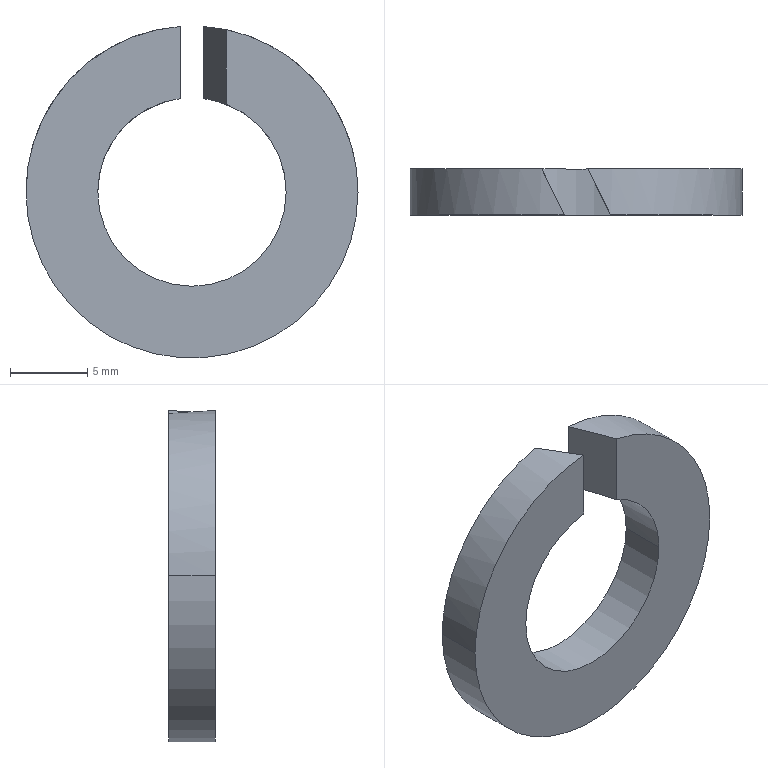Part | STEP file | ZZ24-M12 | 1 solid | 10 faces | box 21.5 x 3 x 21.473 mm | volume 696.301 mm3 | cylinder 6 | plane 4 | commonest cylinder face diameters 12.2 x3 21.5 x3
STEP:
#1=CARTESIAN_POINT('',(0.,0.,0.));
#2=DIRECTION('',(0.,0.,1.));
#3=DIRECTION('',(1.,0.,0.));
#4=AXIS2_PLACEMENT_3D('',#1,#2,#3);
#5=CARTESIAN_POINT('',(2.232,0.,5.677));
#6=VERTEX_POINT('',#5);
#7=CARTESIAN_POINT('',(0.7684,3.,6.051));
#8=VERTEX_POINT('',#7);
#9=CARTESIAN_POINT('',(2.232,0.,5.677));
#10=CARTESIAN_POINT('',(1.761,0.9656,5.862));
#11=CARTESIAN_POINT('',(1.27,1.971,5.988));
#12=CARTESIAN_POINT('',(0.7684,3.,6.051));
#13=(BOUNDED_CURVE()B_SPLINE_CURVE(3,(#9,#10,#11,#12),.UNSPECIFIED.,.F.,.F.)B_SPLINE_CURVE_WITH_KNOTS((4,4),(1.196,1.444),.PIECEWISE_BEZIER_KNOTS.)CURVE()GEOMETRIC_REPRESENTATION_ITEM()RATIONAL_B_SPLINE_CURVE((1.,0.9949,0.9949,1.))REPRESENTATION_ITEM(''));
#14=CARTESIAN_POINT('',(0.,3.,0.));
#15=DIRECTION('',(0.,-1.,0.));
#16=DIRECTION('',(-1.,0.,0.001512));
#17=AXIS2_PLACEMENT_3D('',#14,#15,#16);
#18=CYLINDRICAL_SURFACE('',#17,6.1);
#19=CARTESIAN_POINT('',(4.339,3.));
#20=CARTESIAN_POINT('',(4.343,2.956));
#21=CARTESIAN_POINT('',(4.351,2.869));
#22=CARTESIAN_POINT('',(4.362,2.737));
#23=CARTESIAN_POINT('',(4.373,2.604));
#24=CARTESIAN_POINT('',(4.384,2.471));
#25=CARTESIAN_POINT('',(4.396,2.337));
#26=CARTESIAN_POINT('',(4.407,2.203));
#27=CARTESIAN_POINT('',(4.418,2.068));
#28=CARTESIAN_POINT('',(4.43,1.933));
#29=CARTESIAN_POINT('',(4.441,1.797));
#30=CARTESIAN_POINT('',(4.452,1.661));
#31=CARTESIAN_POINT('',(4.463,1.524));
#32=CARTESIAN_POINT('',(4.475,1.387));
#33=CARTESIAN_POINT('',(4.486,1.249));
#34=CARTESIAN_POINT('',(4.497,1.112));
#35=CARTESIAN_POINT('',(4.509,0.9734));
#36=CARTESIAN_POINT('',(4.52,0.835));
#37=CARTESIAN_POINT('',(4.531,0.6964));
#38=CARTESIAN_POINT('',(4.543,0.5575));
#39=CARTESIAN_POINT('',(4.554,0.4183));
#40=CARTESIAN_POINT('',(4.565,0.2791));
#41=CARTESIAN_POINT('',(4.576,0.1396));
#42=CARTESIAN_POINT('',(4.584,0.04654));
#43=CARTESIAN_POINT('',(4.588,0.));
#44=B_SPLINE_CURVE_WITH_KNOTS('',3,(#19,#20,#21,#22,#23,#24,#25,#26,#27,#28,#29,#30,#31,#32,#33,#34,#35,#36,#37,#38,#39,#40,#41,#42,#43),.UNSPECIFIED.,.F.,.F.,(4,1,1,1,1,1,1,1,1,1,1,1,1,1,1,1,1,1,1,1,1,1,4),(1.196,1.208,1.219,1.23,1.241,1.253,1.264,1.275,1.287,1.298,1.309,1.32,1.332,1.343,1.354,1.366,1.377,1.388,1.399,1.411,1.422,1.433,1.444),.QUASI_UNIFORM_KNOTS.);
#45=(GEOMETRIC_REPRESENTATION_CONTEXT(2)PARAMETRIC_REPRESENTATION_CONTEXT()REPRESENTATION_CONTEXT('',''));
#46=DEFINITIONAL_REPRESENTATION('',(#44),#45);
#47=PCURVE('',#18,#46);
#48=CARTESIAN_POINT('',(2.232,0.,10.75));
#49=DIRECTION('',(-0.8988,-0.4384,0.));
#50=DIRECTION('',(0.4384,-0.8988,0.));
#51=AXIS2_PLACEMENT_3D('',#48,#49,#50);
#52=PLANE('',#51);
#53=CARTESIAN_POINT('',(0.,-5.073));
#54=CARTESIAN_POINT('',(-1.074,-4.888));
#55=CARTESIAN_POINT('',(-2.193,-4.762));
#56=CARTESIAN_POINT('',(-3.338,-4.699));
#57=(BOUNDED_CURVE()B_SPLINE_CURVE(3,(#53,#54,#55,#56),.UNSPECIFIED.,.F.,.F.)B_SPLINE_CURVE_WITH_KNOTS((4,4),(1.196,1.444),.PIECEWISE_BEZIER_KNOTS.)CURVE()GEOMETRIC_REPRESENTATION_ITEM()RATIONAL_B_SPLINE_CURVE((1.,0.9949,0.9949,1.))REPRESENTATION_ITEM(''));
#58=(GEOMETRIC_REPRESENTATION_CONTEXT(2)PARAMETRIC_REPRESENTATION_CONTEXT()REPRESENTATION_CONTEXT('',''));
#59=DEFINITIONAL_REPRESENTATION('',(#57),#58);
#60=PCURVE('',#52,#59);
#61=SURFACE_CURVE('',#13,(#47,#60),.PCURVE_S1.);
#62=EDGE_CURVE('',#6,#8,#61,.T.);
#63=ORIENTED_EDGE('',*,*,#62,.F.);
#64=CARTESIAN_POINT('',(6.1,0.,-0.009225));
#65=VERTEX_POINT('',#64);
#66=CARTESIAN_POINT('',(0.,0.,0.));
#67=DIRECTION('',(0.,1.,0.));
#68=DIRECTION('',(1.,0.,-0.001512));
#69=AXIS2_PLACEMENT_3D('',#66,#67,#68);
#70=CIRCLE('',#69,6.1);
#71=CARTESIAN_POINT('',(9.425,3.));
#72=DIRECTION('',(-1.,0.));
#73=VECTOR('',#72,1.);
#74=LINE('',#71,#73);
#75=(GEOMETRIC_REPRESENTATION_CONTEXT(2)PARAMETRIC_REPRESENTATION_CONTEXT()REPRESENTATION_CONTEXT('',''));
#76=DEFINITIONAL_REPRESENTATION('',(#74),#75);
#77=PCURVE('',#18,#76);
#78=CARTESIAN_POINT('',(0.,0.,0.));
#79=DIRECTION('',(0.,-1.,0.));
#80=DIRECTION('',(-1.,0.,0.001512));
#81=AXIS2_PLACEMENT_3D('',#78,#79,#80);
#82=PLANE('',#81);
#83=CARTESIAN_POINT('',(-6.1,0.));
#84=CARTESIAN_POINT('',(-6.1,10.566));
#85=CARTESIAN_POINT('',(3.05,5.283));
#86=CARTESIAN_POINT('',(12.2,0.));
#87=CARTESIAN_POINT('',(3.05,-5.283));
#88=CARTESIAN_POINT('',(-6.1,-10.566));
#89=CARTESIAN_POINT('',(-6.1,0.));
#90=(BOUNDED_CURVE()B_SPLINE_CURVE(2,(#83,#84,#85,#86,#87,#88,#89),.UNSPECIFIED.,.T.,.F.)B_SPLINE_CURVE_WITH_KNOTS((1,2,2,2,2,1),(-2.094,0.,2.094,4.189,6.283,8.378),.UNSPECIFIED.)CURVE()GEOMETRIC_REPRESENTATION_ITEM()RATIONAL_B_SPLINE_CURVE((1.,0.5,1.,0.5,1.,0.5,1.))REPRESENTATION_ITEM(''));
#91=(GEOMETRIC_REPRESENTATION_CONTEXT(2)PARAMETRIC_REPRESENTATION_CONTEXT()REPRESENTATION_CONTEXT('',''));
#92=DEFINITIONAL_REPRESENTATION('',(#90),#91);
#93=PCURVE('',#82,#92);
#94=SURFACE_CURVE('',#70,(#77,#93),.PCURVE_S1.);
#95=EDGE_CURVE('',#6,#65,#94,.T.);
#96=ORIENTED_EDGE('',*,*,#95,.T.);
#97=CARTESIAN_POINT('',(6.1,3.,-0.009225));
#98=VERTEX_POINT('',#97);
#99=CARTESIAN_POINT('',(6.1,3.,-0.009225));
#100=DIRECTION('',(0.,-1.,0.));
#101=VECTOR('',#100,1.);
#102=LINE('',#99,#101);
#103=CARTESIAN_POINT('',(3.142,0.));
#104=DIRECTION('',(0.,1.));
#105=VECTOR('',#104,1.);
#106=LINE('',#103,#105);
#107=(GEOMETRIC_REPRESENTATION_CONTEXT(2)PARAMETRIC_REPRESENTATION_CONTEXT()REPRESENTATION_CONTEXT('',''));
#108=DEFINITIONAL_REPRESENTATION('',(#106),#107);
#109=PCURVE('',#18,#108);
#110=CARTESIAN_POINT('',(0.,3.,0.));
#111=DIRECTION('',(0.,-1.,0.));
#112=DIRECTION('',(-1.,0.,0.001512));
#113=AXIS2_PLACEMENT_3D('',#110,#111,#112);
#114=CYLINDRICAL_SURFACE('',#113,6.1);
#115=CARTESIAN_POINT('',(3.142,0.));
#116=DIRECTION('',(0.,1.));
#117=VECTOR('',#116,1.);
#118=LINE('',#115,#117);
#119=(GEOMETRIC_REPRESENTATION_CONTEXT(2)PARAMETRIC_REPRESENTATION_CONTEXT()REPRESENTATION_CONTEXT('',''));
#120=DEFINITIONAL_REPRESENTATION('',(#118),#119);
#121=PCURVE('',#114,#120);
#122=SURFACE_CURVE('',#102,(#109,#121),.PCURVE_S1.);
#123=EDGE_CURVE('',#98,#65,#122,.T.);
#124=ORIENTED_EDGE('',*,*,#123,.F.);
#125=CARTESIAN_POINT('',(0.,3.,0.));
#126=DIRECTION('',(0.,-1.,0.));
#127=DIRECTION('',(-1.,0.,0.001512));
#128=AXIS2_PLACEMENT_3D('',#125,#126,#127);
#129=CIRCLE('',#128,6.1);
#130=CARTESIAN_POINT('',(0.,0.));
#131=DIRECTION('',(1.,0.));
#132=VECTOR('',#131,1.);
#133=LINE('',#130,#132);
#134=(GEOMETRIC_REPRESENTATION_CONTEXT(2)PARAMETRIC_REPRESENTATION_CONTEXT()REPRESENTATION_CONTEXT('',''));
#135=DEFINITIONAL_REPRESENTATION('',(#133),#134);
#136=PCURVE('',#18,#135);
#137=CARTESIAN_POINT('',(0.,3.,0.));
#138=DIRECTION('',(0.,1.,0.));
#139=DIRECTION('',(1.,0.,-0.001512));
#140=AXIS2_PLACEMENT_3D('',#137,#138,#139);
#141=PLANE('',#140);
#142=CARTESIAN_POINT('',(-6.1,0.));
#143=CARTESIAN_POINT('',(-6.1,10.566));
#144=CARTESIAN_POINT('',(3.05,5.283));
#145=CARTESIAN_POINT('',(12.2,0.));
#146=CARTESIAN_POINT('',(3.05,-5.283));
#147=CARTESIAN_POINT('',(-6.1,-10.566));
#148=CARTESIAN_POINT('',(-6.1,0.));
#149=(BOUNDED_CURVE()B_SPLINE_CURVE(2,(#142,#143,#144,#145,#146,#147,#148),.UNSPECIFIED.,.T.,.F.)B_SPLINE_CURVE_WITH_KNOTS((1,2,2,2,2,1),(-2.094,0.,2.094,4.189,6.283,8.378),.UNSPECIFIED.)CURVE()GEOMETRIC_REPRESENTATION_ITEM()RATIONAL_B_SPLINE_CURVE((1.,0.5,1.,0.5,1.,0.5,1.))REPRESENTATION_ITEM(''));
#150=(GEOMETRIC_REPRESENTATION_CONTEXT(2)PARAMETRIC_REPRESENTATION_CONTEXT()REPRESENTATION_CONTEXT('',''));
#151=DEFINITIONAL_REPRESENTATION('',(#149),#150);
#152=PCURVE('',#141,#151);
#153=SURFACE_CURVE('',#129,(#136,#152),.PCURVE_S1.);
#154=EDGE_CURVE('',#98,#8,#153,.T.);
#155=ORIENTED_EDGE('',*,*,#154,.T.);
#156=EDGE_LOOP('',(#63,#96,#124,#155));
#157=FACE_BOUND('',#156,.F.);
#158=ADVANCED_FACE('',(#157),#18,.F.);
#159=CARTESIAN_POINT('',(-6.1,0.,0.009225));
#160=VERTEX_POINT('',#159);
#161=CARTESIAN_POINT('',(0.,0.,0.));
#162=DIRECTION('',(0.,1.,0.));
#163=DIRECTION('',(1.,0.,-0.001512));
#164=AXIS2_PLACEMENT_3D('',#161,#162,#163);
#165=CIRCLE('',#164,6.1);
#166=CARTESIAN_POINT('',(3.142,3.));
#167=DIRECTION('',(-1.,0.));
#168=VECTOR('',#167,1.);
#169=LINE('',#166,#168);
#170=(GEOMETRIC_REPRESENTATION_CONTEXT(2)PARAMETRIC_REPRESENTATION_CONTEXT()REPRESENTATION_CONTEXT('',''));
#171=DEFINITIONAL_REPRESENTATION('',(#169),#170);
#172=PCURVE('',#114,#171);
#173=CARTESIAN_POINT('',(-6.1,0.));
#174=CARTESIAN_POINT('',(-6.1,10.566));
#175=CARTESIAN_POINT('',(3.05,5.283));
#176=CARTESIAN_POINT('',(12.2,0.));
#177=CARTESIAN_POINT('',(3.05,-5.283));
#178=CARTESIAN_POINT('',(-6.1,-10.566));
#179=CARTESIAN_POINT('',(-6.1,0.));
#180=(BOUNDED_CURVE()B_SPLINE_CURVE(2,(#173,#174,#175,#176,#177,#178,#179),.UNSPECIFIED.,.T.,.F.)B_SPLINE_CURVE_WITH_KNOTS((1,2,2,2,2,1),(-2.094,0.,2.094,4.189,6.283,8.378),.UNSPECIFIED.)CURVE()GEOMETRIC_REPRESENTATION_ITEM()RATIONAL_B_SPLINE_CURVE((1.,0.5,1.,0.5,1.,0.5,1.))REPRESENTATION_ITEM(''));
#181=(GEOMETRIC_REPRESENTATION_CONTEXT(2)PARAMETRIC_REPRESENTATION_CONTEXT()REPRESENTATION_CONTEXT('',''));
#182=DEFINITIONAL_REPRESENTATION('',(#180),#181);
#183=PCURVE('',#82,#182);
#184=SURFACE_CURVE('',#165,(#172,#183),.PCURVE_S1.);
#185=EDGE_CURVE('',#65,#160,#184,.T.);
#186=ORIENTED_EDGE('',*,*,#185,.T.);
#187=CARTESIAN_POINT('',(-6.1,3.,0.009225));
#188=VERTEX_POINT('',#187);
#189=CARTESIAN_POINT('',(-6.1,3.,0.009225));
#190=DIRECTION('',(0.,-1.,0.));
#191=VECTOR('',#190,1.);
#192=LINE('',#189,#191);
#193=CARTESIAN_POINT('',(0.,0.));
#194=DIRECTION('',(0.,1.));
#195=VECTOR('',#194,1.);
#196=LINE('',#193,#195);
#197=(GEOMETRIC_REPRESENTATION_CONTEXT(2)PARAMETRIC_REPRESENTATION_CONTEXT()REPRESENTATION_CONTEXT('',''));
#198=DEFINITIONAL_REPRESENTATION('',(#196),#197);
#199=PCURVE('',#114,#198);
#200=CARTESIAN_POINT('',(0.,3.,0.));
#201=DIRECTION('',(0.,-1.,0.));
#202=DIRECTION('',(-1.,0.,0.001512));
#203=AXIS2_PLACEMENT_3D('',#200,#201,#202);
#204=CYLINDRICAL_SURFACE('',#203,6.1);
#205=CARTESIAN_POINT('',(6.283,0.));
#206=DIRECTION('',(0.,1.));
#207=VECTOR('',#206,1.);
#208=LINE('',#205,#207);
#209=(GEOMETRIC_REPRESENTATION_CONTEXT(2)PARAMETRIC_REPRESENTATION_CONTEXT()REPRESENTATION_CONTEXT('',''));
#210=DEFINITIONAL_REPRESENTATION('',(#208),#209);
#211=PCURVE('',#204,#210);
#212=SURFACE_CURVE('',#192,(#199,#211),.PCURVE_S1.);
#213=EDGE_CURVE('',#188,#160,#212,.T.);
#214=ORIENTED_EDGE('',*,*,#213,.F.);
#215=CARTESIAN_POINT('',(0.,3.,0.));
#216=DIRECTION('',(0.,-1.,0.));
#217=DIRECTION('',(-1.,0.,0.001512));
#218=AXIS2_PLACEMENT_3D('',#215,#216,#217);
#219=CIRCLE('',#218,6.1);
#220=CARTESIAN_POINT('',(0.,0.));
#221=DIRECTION('',(1.,0.));
#222=VECTOR('',#221,1.);
#223=LINE('',#220,#222);
#224=(GEOMETRIC_REPRESENTATION_CONTEXT(2)PARAMETRIC_REPRESENTATION_CONTEXT()REPRESENTATION_CONTEXT('',''));
#225=DEFINITIONAL_REPRESENTATION('',(#223),#224);
#226=PCURVE('',#114,#225);
#227=CARTESIAN_POINT('',(-6.1,0.));
#228=CARTESIAN_POINT('',(-6.1,10.566));
#229=CARTESIAN_POINT('',(3.05,5.283));
#230=CARTESIAN_POINT('',(12.2,0.));
#231=CARTESIAN_POINT('',(3.05,-5.283));
#232=CARTESIAN_POINT('',(-6.1,-10.566));
#233=CARTESIAN_POINT('',(-6.1,0.));
#234=(BOUNDED_CURVE()B_SPLINE_CURVE(2,(#227,#228,#229,#230,#231,#232,#233),.UNSPECIFIED.,.T.,.F.)B_SPLINE_CURVE_WITH_KNOTS((1,2,2,2,2,1),(-2.094,0.,2.094,4.189,6.283,8.378),.UNSPECIFIED.)CURVE()GEOMETRIC_REPRESENTATION_ITEM()RATIONAL_B_SPLINE_CURVE((1.,0.5,1.,0.5,1.,0.5,1.))REPRESENTATION_ITEM(''));
#235=(GEOMETRIC_REPRESENTATION_CONTEXT(2)PARAMETRIC_REPRESENTATION_CONTEXT()REPRESENTATION_CONTEXT('',''));
#236=DEFINITIONAL_REPRESENTATION('',(#234),#235);
#237=PCURVE('',#141,#236);
#238=SURFACE_CURVE('',#219,(#226,#237),.PCURVE_S1.);
#239=EDGE_CURVE('',#188,#98,#238,.T.);
#240=ORIENTED_EDGE('',*,*,#239,.T.);
#241=ORIENTED_EDGE('',*,*,#123,.T.);
#242=EDGE_LOOP('',(#186,#214,#240,#241));
#243=FACE_BOUND('',#242,.F.);
#244=ADVANCED_FACE('',(#243),#114,.F.);
#245=CARTESIAN_POINT('',(-10.75,3.,0.01626));
#246=VERTEX_POINT('',#245);
#247=CARTESIAN_POINT('',(10.75,3.,-0.01626));
#248=VERTEX_POINT('',#247);
#249=CARTESIAN_POINT('',(0.,3.,0.));
#250=DIRECTION('',(0.,-1.,0.));
#251=DIRECTION('',(-1.,0.,0.001512));
#252=AXIS2_PLACEMENT_3D('',#249,#250,#251);
#253=CIRCLE('',#252,10.75);
#254=CARTESIAN_POINT('',(0.,3.,0.));
#255=DIRECTION('',(0.,-1.,0.));
#256=DIRECTION('',(-1.,0.,0.001512));
#257=AXIS2_PLACEMENT_3D('',#254,#255,#256);
#258=CYLINDRICAL_SURFACE('',#257,10.75);
#259=CARTESIAN_POINT('',(0.,0.));
#260=DIRECTION('',(1.,0.));
#261=VECTOR('',#260,1.);
#262=LINE('',#259,#261);
#263=(GEOMETRIC_REPRESENTATION_CONTEXT(2)PARAMETRIC_REPRESENTATION_CONTEXT()REPRESENTATION_CONTEXT('',''));
#264=DEFINITIONAL_REPRESENTATION('',(#262),#263);
#265=PCURVE('',#258,#264);
#266=CARTESIAN_POINT('',(-10.75,0.));
#267=CARTESIAN_POINT('',(-10.75,18.62));
#268=CARTESIAN_POINT('',(5.375,9.31));
#269=CARTESIAN_POINT('',(21.5,0.));
#270=CARTESIAN_POINT('',(5.375,-9.31));
#271=CARTESIAN_POINT('',(-10.75,-18.62));
#272=CARTESIAN_POINT('',(-10.75,0.));
#273=(BOUNDED_CURVE()B_SPLINE_CURVE(2,(#266,#267,#268,#269,#270,#271,#272),.UNSPECIFIED.,.T.,.F.)B_SPLINE_CURVE_WITH_KNOTS((1,2,2,2,2,1),(-2.094,0.,2.094,4.189,6.283,8.378),.UNSPECIFIED.)CURVE()GEOMETRIC_REPRESENTATION_ITEM()RATIONAL_B_SPLINE_CURVE((1.,0.5,1.,0.5,1.,0.5,1.))REPRESENTATION_ITEM(''));
#274=(GEOMETRIC_REPRESENTATION_CONTEXT(2)PARAMETRIC_REPRESENTATION_CONTEXT()REPRESENTATION_CONTEXT('',''));
#275=DEFINITIONAL_REPRESENTATION('',(#273),#274);
#276=PCURVE('',#141,#275);
#277=SURFACE_CURVE('',#253,(#265,#276),.PCURVE_S1.);
#278=EDGE_CURVE('',#246,#248,#277,.T.);
#279=ORIENTED_EDGE('',*,*,#278,.T.);
#280=CARTESIAN_POINT('',(10.75,0.,-0.01626));
#281=VERTEX_POINT('',#280);
#282=CARTESIAN_POINT('',(10.75,3.,-0.01626));
#283=DIRECTION('',(0.,-1.,0.));
#284=VECTOR('',#283,1.);
#285=LINE('',#282,#284);
#286=CARTESIAN_POINT('',(3.142,0.));
#287=DIRECTION('',(0.,1.));
#288=VECTOR('',#287,1.);
#289=LINE('',#286,#288);
#290=(GEOMETRIC_REPRESENTATION_CONTEXT(2)PARAMETRIC_REPRESENTATION_CONTEXT()REPRESENTATION_CONTEXT('',''));
#291=DEFINITIONAL_REPRESENTATION('',(#289),#290);
#292=PCURVE('',#258,#291);
#293=CARTESIAN_POINT('',(0.,3.,0.));
#294=DIRECTION('',(0.,-1.,0.));
#295=DIRECTION('',(-1.,0.,0.001512));
#296=AXIS2_PLACEMENT_3D('',#293,#294,#295);
#297=CYLINDRICAL_SURFACE('',#296,10.75);
#298=CARTESIAN_POINT('',(3.142,0.));
#299=DIRECTION('',(0.,1.));
#300=VECTOR('',#299,1.);
#301=LINE('',#298,#300);
#302=(GEOMETRIC_REPRESENTATION_CONTEXT(2)PARAMETRIC_REPRESENTATION_CONTEXT()REPRESENTATION_CONTEXT('',''));
#303=DEFINITIONAL_REPRESENTATION('',(#301),#302);
#304=PCURVE('',#297,#303);
#305=SURFACE_CURVE('',#285,(#292,#304),.PCURVE_S1.);
#306=EDGE_CURVE('',#248,#281,#305,.T.);
#307=ORIENTED_EDGE('',*,*,#306,.T.);
#308=CARTESIAN_POINT('',(-10.75,0.,0.01626));
#309=VERTEX_POINT('',#308);
#310=CARTESIAN_POINT('',(0.,0.,0.));
#311=DIRECTION('',(0.,1.,0.));
#312=DIRECTION('',(1.,0.,-0.001512));
#313=AXIS2_PLACEMENT_3D('',#310,#311,#312);
#314=CIRCLE('',#313,10.75);
#315=CARTESIAN_POINT('',(3.142,3.));
#316=DIRECTION('',(-1.,0.));
#317=VECTOR('',#316,1.);
#318=LINE('',#315,#317);
#319=(GEOMETRIC_REPRESENTATION_CONTEXT(2)PARAMETRIC_REPRESENTATION_CONTEXT()REPRESENTATION_CONTEXT('',''));
#320=DEFINITIONAL_REPRESENTATION('',(#318),#319);
#321=PCURVE('',#258,#320);
#322=CARTESIAN_POINT('',(-10.75,0.));
#323=CARTESIAN_POINT('',(-10.75,18.62));
#324=CARTESIAN_POINT('',(5.375,9.31));
#325=CARTESIAN_POINT('',(21.5,0.));
#326=CARTESIAN_POINT('',(5.375,-9.31));
#327=CARTESIAN_POINT('',(-10.75,-18.62));
#328=CARTESIAN_POINT('',(-10.75,0.));
#329=(BOUNDED_CURVE()B_SPLINE_CURVE(2,(#322,#323,#324,#325,#326,#327,#328),.UNSPECIFIED.,.T.,.F.)B_SPLINE_CURVE_WITH_KNOTS((1,2,2,2,2,1),(-2.094,0.,2.094,4.189,6.283,8.378),.UNSPECIFIED.)CURVE()GEOMETRIC_REPRESENTATION_ITEM()RATIONAL_B_SPLINE_CURVE((1.,0.5,1.,0.5,1.,0.5,1.))REPRESENTATION_ITEM(''));
#330=(GEOMETRIC_REPRESENTATION_CONTEXT(2)PARAMETRIC_REPRESENTATION_CONTEXT()REPRESENTATION_CONTEXT('',''));
#331=DEFINITIONAL_REPRESENTATION('',(#329),#330);
#332=PCURVE('',#82,#331);
#333=SURFACE_CURVE('',#314,(#321,#332),.PCURVE_S1.);
#334=EDGE_CURVE('',#281,#309,#333,.T.);
#335=ORIENTED_EDGE('',*,*,#334,.T.);
#336=CARTESIAN_POINT('',(-10.75,3.,0.01626));
#337=DIRECTION('',(0.,-1.,0.));
#338=VECTOR('',#337,1.);
#339=LINE('',#336,#338);
#340=CARTESIAN_POINT('',(0.,0.));
#341=DIRECTION('',(0.,1.));
#342=VECTOR('',#341,1.);
#343=LINE('',#340,#342);
#344=(GEOMETRIC_REPRESENTATION_CONTEXT(2)PARAMETRIC_REPRESENTATION_CONTEXT()REPRESENTATION_CONTEXT('',''));
#345=DEFINITIONAL_REPRESENTATION('',(#343),#344);
#346=PCURVE('',#258,#345);
#347=CARTESIAN_POINT('',(0.,3.,0.));
#348=DIRECTION('',(0.,-1.,0.));
#349=DIRECTION('',(-1.,0.,0.001512));
#350=AXIS2_PLACEMENT_3D('',#347,#348,#349);
#351=CYLINDRICAL_SURFACE('',#350,10.75);
#352=CARTESIAN_POINT('',(6.283,0.));
#353=DIRECTION('',(0.,1.));
#354=VECTOR('',#353,1.);
#355=LINE('',#352,#354);
#356=(GEOMETRIC_REPRESENTATION_CONTEXT(2)PARAMETRIC_REPRESENTATION_CONTEXT()REPRESENTATION_CONTEXT('',''));
#357=DEFINITIONAL_REPRESENTATION('',(#355),#356);
#358=PCURVE('',#351,#357);
#359=SURFACE_CURVE('',#339,(#346,#358),.PCURVE_S1.);
#360=EDGE_CURVE('',#246,#309,#359,.T.);
#361=ORIENTED_EDGE('',*,*,#360,.F.);
#362=EDGE_LOOP('',(#279,#307,#335,#361));
#363=FACE_BOUND('',#362,.T.);
#364=ADVANCED_FACE('',(#363),#258,.T.);
#365=CARTESIAN_POINT('',(-2.232,3.,10.516));
#366=VERTEX_POINT('',#365);
#367=CARTESIAN_POINT('',(0.,3.,0.));
#368=DIRECTION('',(0.,-1.,0.));
#369=DIRECTION('',(-1.,0.,0.001512));
#370=AXIS2_PLACEMENT_3D('',#367,#368,#369);
#371=CIRCLE('',#370,10.75);
#372=CARTESIAN_POINT('',(0.,0.));
#373=DIRECTION('',(1.,0.));
#374=VECTOR('',#373,1.);
#375=LINE('',#372,#374);
#376=(GEOMETRIC_REPRESENTATION_CONTEXT(2)PARAMETRIC_REPRESENTATION_CONTEXT()REPRESENTATION_CONTEXT('',''));
#377=DEFINITIONAL_REPRESENTATION('',(#375),#376);
#378=PCURVE('',#351,#377);
#379=CARTESIAN_POINT('',(-10.75,0.));
#380=CARTESIAN_POINT('',(-10.75,18.62));
#381=CARTESIAN_POINT('',(5.375,9.31));
#382=CARTESIAN_POINT('',(21.5,0.));
#383=CARTESIAN_POINT('',(5.375,-9.31));
#384=CARTESIAN_POINT('',(-10.75,-18.62));
#385=CARTESIAN_POINT('',(-10.75,0.));
#386=(BOUNDED_CURVE()B_SPLINE_CURVE(2,(#379,#380,#381,#382,#383,#384,#385),.UNSPECIFIED.,.T.,.F.)B_SPLINE_CURVE_WITH_KNOTS((1,2,2,2,2,1),(-2.094,0.,2.094,4.189,6.283,8.378),.UNSPECIFIED.)CURVE()GEOMETRIC_REPRESENTATION_ITEM()RATIONAL_B_SPLINE_CURVE((1.,0.5,1.,0.5,1.,0.5,1.))REPRESENTATION_ITEM(''));
#387=(GEOMETRIC_REPRESENTATION_CONTEXT(2)PARAMETRIC_REPRESENTATION_CONTEXT()REPRESENTATION_CONTEXT('',''));
#388=DEFINITIONAL_REPRESENTATION('',(#386),#387);
#389=PCURVE('',#141,#388);
#390=SURFACE_CURVE('',#371,(#378,#389),.PCURVE_S1.);
#391=EDGE_CURVE('',#366,#246,#390,.T.);
#392=ORIENTED_EDGE('',*,*,#391,.T.);
#393=ORIENTED_EDGE('',*,*,#360,.T.);
#394=CARTESIAN_POINT('',(-0.7684,0.,10.723));
#395=VERTEX_POINT('',#394);
#396=CARTESIAN_POINT('',(0.,0.,0.));
#397=DIRECTION('',(0.,1.,0.));
#398=DIRECTION('',(1.,0.,-0.001512));
#399=AXIS2_PLACEMENT_3D('',#396,#397,#398);
#400=CIRCLE('',#399,10.75);
#401=CARTESIAN_POINT('',(9.425,3.));
#402=DIRECTION('',(-1.,0.));
#403=VECTOR('',#402,1.);
#404=LINE('',#401,#403);
#405=(GEOMETRIC_REPRESENTATION_CONTEXT(2)PARAMETRIC_REPRESENTATION_CONTEXT()REPRESENTATION_CONTEXT('',''));
#406=DEFINITIONAL_REPRESENTATION('',(#404),#405);
#407=PCURVE('',#351,#406);
#408=CARTESIAN_POINT('',(-10.75,0.));
#409=CARTESIAN_POINT('',(-10.75,18.62));
#410=CARTESIAN_POINT('',(5.375,9.31));
#411=CARTESIAN_POINT('',(21.5,0.));
#412=CARTESIAN_POINT('',(5.375,-9.31));
#413=CARTESIAN_POINT('',(-10.75,-18.62));
#414=CARTESIAN_POINT('',(-10.75,0.));
#415=(BOUNDED_CURVE()B_SPLINE_CURVE(2,(#408,#409,#410,#411,#412,#413,#414),.UNSPECIFIED.,.T.,.F.)B_SPLINE_CURVE_WITH_KNOTS((1,2,2,2,2,1),(-2.094,0.,2.094,4.189,6.283,8.378),.UNSPECIFIED.)CURVE()GEOMETRIC_REPRESENTATION_ITEM()RATIONAL_B_SPLINE_CURVE((1.,0.5,1.,0.5,1.,0.5,1.))REPRESENTATION_ITEM(''));
#416=(GEOMETRIC_REPRESENTATION_CONTEXT(2)PARAMETRIC_REPRESENTATION_CONTEXT()REPRESENTATION_CONTEXT('',''));
#417=DEFINITIONAL_REPRESENTATION('',(#415),#416);
#418=PCURVE('',#82,#417);
#419=SURFACE_CURVE('',#400,(#407,#418),.PCURVE_S1.);
#420=EDGE_CURVE('',#309,#395,#419,.T.);
#421=ORIENTED_EDGE('',*,*,#420,.T.);
#422=CARTESIAN_POINT('',(-0.7684,0.,10.723));
#423=CARTESIAN_POINT('',(-1.26,1.009,10.687));
#424=CARTESIAN_POINT('',(-1.749,2.011,10.618));
#425=CARTESIAN_POINT('',(-2.232,3.,10.516));
#426=(BOUNDED_CURVE()B_SPLINE_CURVE(3,(#422,#423,#424,#425),.UNSPECIFIED.,.F.,.F.)B_SPLINE_CURVE_WITH_KNOTS((4,4),(1.642,1.78),.PIECEWISE_BEZIER_KNOTS.)CURVE()GEOMETRIC_REPRESENTATION_ITEM()RATIONAL_B_SPLINE_CURVE((1.,0.9984,0.9984,1.))REPRESENTATION_ITEM(''));
#427=CARTESIAN_POINT('',(4.785,3.));
#428=CARTESIAN_POINT('',(4.788,2.954));
#429=CARTESIAN_POINT('',(4.792,2.863));
#430=CARTESIAN_POINT('',(4.798,2.725));
#431=CARTESIAN_POINT('',(4.804,2.588));
#432=CARTESIAN_POINT('',(4.81,2.451));
#433=CARTESIAN_POINT('',(4.817,2.314));
#434=CARTESIAN_POINT('',(4.823,2.177));
#435=CARTESIAN_POINT('',(4.829,2.04));
#436=CARTESIAN_POINT('',(4.835,1.903));
#437=CARTESIAN_POINT('',(4.842,1.766));
#438=CARTESIAN_POINT('',(4.848,1.629));
#439=CARTESIAN_POINT('',(4.854,1.493));
#440=CARTESIAN_POINT('',(4.86,1.356));
#441=CARTESIAN_POINT('',(4.867,1.22));
#442=CARTESIAN_POINT('',(4.873,1.084));
#443=CARTESIAN_POINT('',(4.879,0.9476));
#444=CARTESIAN_POINT('',(4.886,0.8117));
#445=CARTESIAN_POINT('',(4.892,0.676));
#446=CARTESIAN_POINT('',(4.898,0.5404));
#447=CARTESIAN_POINT('',(4.904,0.405));
#448=CARTESIAN_POINT('',(4.911,0.2698));
#449=CARTESIAN_POINT('',(4.917,0.1348));
#450=CARTESIAN_POINT('',(4.921,0.04491));
#451=CARTESIAN_POINT('',(4.923,0.));
#452=B_SPLINE_CURVE_WITH_KNOTS('',3,(#427,#428,#429,#430,#431,#432,#433,#434,#435,#436,#437,#438,#439,#440,#441,#442,#443,#444,#445,#446,#447,#448,#449,#450,#451),.UNSPECIFIED.,.F.,.F.,(4,1,1,1,1,1,1,1,1,1,1,1,1,1,1,1,1,1,1,1,1,1,4),(1.642,1.649,1.655,1.661,1.667,1.674,1.68,1.686,1.692,1.699,1.705,1.711,1.717,1.724,1.73,1.736,1.742,1.749,1.755,1.761,1.767,1.774,1.78),.QUASI_UNIFORM_KNOTS.);
#453=(GEOMETRIC_REPRESENTATION_CONTEXT(2)PARAMETRIC_REPRESENTATION_CONTEXT()REPRESENTATION_CONTEXT('',''));
#454=DEFINITIONAL_REPRESENTATION('',(#452),#453);
#455=PCURVE('',#351,#454);
#456=CARTESIAN_POINT('',(-2.232,3.,10.75));
#457=DIRECTION('',(0.8988,0.4384,0.));
#458=DIRECTION('',(-0.4384,0.8988,0.));
#459=AXIS2_PLACEMENT_3D('',#456,#457,#458);
#460=PLANE('',#459);
#461=CARTESIAN_POINT('',(-3.338,-0.0275));
#462=CARTESIAN_POINT('',(-2.215,-0.06276));
#463=CARTESIAN_POINT('',(-1.101,-0.1318));
#464=CARTESIAN_POINT('',(0.,-0.2342));
#465=(BOUNDED_CURVE()B_SPLINE_CURVE(3,(#461,#462,#463,#464),.UNSPECIFIED.,.F.,.F.)B_SPLINE_CURVE_WITH_KNOTS((4,4),(1.642,1.78),.PIECEWISE_BEZIER_KNOTS.)CURVE()GEOMETRIC_REPRESENTATION_ITEM()RATIONAL_B_SPLINE_CURVE((1.,0.9984,0.9984,1.))REPRESENTATION_ITEM(''));
#466=(GEOMETRIC_REPRESENTATION_CONTEXT(2)PARAMETRIC_REPRESENTATION_CONTEXT()REPRESENTATION_CONTEXT('',''));
#467=DEFINITIONAL_REPRESENTATION('',(#465),#466);
#468=PCURVE('',#460,#467);
#469=SURFACE_CURVE('',#426,(#455,#468),.PCURVE_S1.);
#470=EDGE_CURVE('',#395,#366,#469,.T.);
#471=ORIENTED_EDGE('',*,*,#470,.T.);
#472=EDGE_LOOP('',(#392,#393,#421,#471));
#473=FACE_BOUND('',#472,.T.);
#474=ADVANCED_FACE('',(#473),#351,.T.);
#475=CARTESIAN_POINT('',(-0.7684,0.,6.051));
#476=VERTEX_POINT('',#475);
#477=CARTESIAN_POINT('',(-0.7684,0.,10.75));
#478=DIRECTION('',(0.,0.,-1.));
#479=VECTOR('',#478,1.);
#480=LINE('',#477,#479);
#481=CARTESIAN_POINT('',(0.7847,-10.749));
#482=DIRECTION('',(-0.001512,1.));
#483=VECTOR('',#482,1.);
#484=LINE('',#481,#483);
#485=(GEOMETRIC_REPRESENTATION_CONTEXT(2)PARAMETRIC_REPRESENTATION_CONTEXT()REPRESENTATION_CONTEXT('',''));
#486=DEFINITIONAL_REPRESENTATION('',(#484),#485);
#487=PCURVE('',#82,#486);
#488=CARTESIAN_POINT('',(-3.338,0.));
#489=DIRECTION('',(0.,-1.));
#490=VECTOR('',#489,1.);
#491=LINE('',#488,#490);
#492=(GEOMETRIC_REPRESENTATION_CONTEXT(2)PARAMETRIC_REPRESENTATION_CONTEXT()REPRESENTATION_CONTEXT('',''));
#493=DEFINITIONAL_REPRESENTATION('',(#491),#492);
#494=PCURVE('',#460,#493);
#495=SURFACE_CURVE('',#480,(#487,#494),.PCURVE_S1.);
#496=EDGE_CURVE('',#395,#476,#495,.T.);
#497=ORIENTED_EDGE('',*,*,#496,.F.);
#498=ORIENTED_EDGE('',*,*,#420,.F.);
#499=ORIENTED_EDGE('',*,*,#334,.F.);
#500=CARTESIAN_POINT('',(2.232,0.,10.516));
#501=VERTEX_POINT('',#500);
#502=CARTESIAN_POINT('',(0.,0.,0.));
#503=DIRECTION('',(0.,1.,0.));
#504=DIRECTION('',(1.,0.,-0.001512));
#505=AXIS2_PLACEMENT_3D('',#502,#503,#504);
#506=CIRCLE('',#505,10.75);
#507=CARTESIAN_POINT('',(-10.75,0.));
#508=CARTESIAN_POINT('',(-10.75,18.62));
#509=CARTESIAN_POINT('',(5.375,9.31));
#510=CARTESIAN_POINT('',(21.5,0.));
#511=CARTESIAN_POINT('',(5.375,-9.31));
#512=CARTESIAN_POINT('',(-10.75,-18.62));
#513=CARTESIAN_POINT('',(-10.75,0.));
#514=(BOUNDED_CURVE()B_SPLINE_CURVE(2,(#507,#508,#509,#510,#511,#512,#513),.UNSPECIFIED.,.T.,.F.)B_SPLINE_CURVE_WITH_KNOTS((1,2,2,2,2,1),(-2.094,0.,2.094,4.189,6.283,8.378),.UNSPECIFIED.)CURVE()GEOMETRIC_REPRESENTATION_ITEM()RATIONAL_B_SPLINE_CURVE((1.,0.5,1.,0.5,1.,0.5,1.))REPRESENTATION_ITEM(''));
#515=(GEOMETRIC_REPRESENTATION_CONTEXT(2)PARAMETRIC_REPRESENTATION_CONTEXT()REPRESENTATION_CONTEXT('',''));
#516=DEFINITIONAL_REPRESENTATION('',(#514),#515);
#517=PCURVE('',#82,#516);
#518=CARTESIAN_POINT('',(9.425,3.));
#519=DIRECTION('',(-1.,0.));
#520=VECTOR('',#519,1.);
#521=LINE('',#518,#520);
#522=(GEOMETRIC_REPRESENTATION_CONTEXT(2)PARAMETRIC_REPRESENTATION_CONTEXT()REPRESENTATION_CONTEXT('',''));
#523=DEFINITIONAL_REPRESENTATION('',(#521),#522);
#524=PCURVE('',#297,#523);
#525=SURFACE_CURVE('',#506,(#517,#524),.PCURVE_S1.);
#526=EDGE_CURVE('',#501,#281,#525,.T.);
#527=ORIENTED_EDGE('',*,*,#526,.F.);
#528=CARTESIAN_POINT('',(2.232,0.,10.75));
#529=DIRECTION('',(0.,0.,-1.));
#530=VECTOR('',#529,1.);
#531=LINE('',#528,#530);
#532=CARTESIAN_POINT('',(-2.215,-10.753));
#533=DIRECTION('',(-0.001512,1.));
#534=VECTOR('',#533,1.);
#535=LINE('',#532,#534);
#536=(GEOMETRIC_REPRESENTATION_CONTEXT(2)PARAMETRIC_REPRESENTATION_CONTEXT()REPRESENTATION_CONTEXT('',''));
#537=DEFINITIONAL_REPRESENTATION('',(#535),#536);
#538=PCURVE('',#82,#537);
#539=CARTESIAN_POINT('',(0.,0.));
#540=DIRECTION('',(0.,-1.));
#541=VECTOR('',#540,1.);
#542=LINE('',#539,#541);
#543=(GEOMETRIC_REPRESENTATION_CONTEXT(2)PARAMETRIC_REPRESENTATION_CONTEXT()REPRESENTATION_CONTEXT('',''));
#544=DEFINITIONAL_REPRESENTATION('',(#542),#543);
#545=PCURVE('',#52,#544);
#546=SURFACE_CURVE('',#531,(#538,#545),.PCURVE_S1.);
#547=EDGE_CURVE('',#501,#6,#546,.T.);
#548=ORIENTED_EDGE('',*,*,#547,.T.);
#549=ORIENTED_EDGE('',*,*,#95,.T.);
#550=ORIENTED_EDGE('',*,*,#185,.T.);
#551=CARTESIAN_POINT('',(0.,0.,0.));
#552=DIRECTION('',(0.,1.,0.));
#553=DIRECTION('',(1.,0.,-0.001512));
#554=AXIS2_PLACEMENT_3D('',#551,#552,#553);
#555=CIRCLE('',#554,6.1);
#556=CARTESIAN_POINT('',(-6.1,0.));
#557=CARTESIAN_POINT('',(-6.1,10.566));
#558=CARTESIAN_POINT('',(3.05,5.283));
#559=CARTESIAN_POINT('',(12.2,0.));
#560=CARTESIAN_POINT('',(3.05,-5.283));
#561=CARTESIAN_POINT('',(-6.1,-10.566));
#562=CARTESIAN_POINT('',(-6.1,0.));
#563=(BOUNDED_CURVE()B_SPLINE_CURVE(2,(#556,#557,#558,#559,#560,#561,#562),.UNSPECIFIED.,.T.,.F.)B_SPLINE_CURVE_WITH_KNOTS((1,2,2,2,2,1),(-2.094,0.,2.094,4.189,6.283,8.378),.UNSPECIFIED.)CURVE()GEOMETRIC_REPRESENTATION_ITEM()RATIONAL_B_SPLINE_CURVE((1.,0.5,1.,0.5,1.,0.5,1.))REPRESENTATION_ITEM(''));
#564=(GEOMETRIC_REPRESENTATION_CONTEXT(2)PARAMETRIC_REPRESENTATION_CONTEXT()REPRESENTATION_CONTEXT('',''));
#565=DEFINITIONAL_REPRESENTATION('',(#563),#564);
#566=PCURVE('',#82,#565);
#567=CARTESIAN_POINT('',(9.425,3.));
#568=DIRECTION('',(-1.,0.));
#569=VECTOR('',#568,1.);
#570=LINE('',#567,#569);
#571=(GEOMETRIC_REPRESENTATION_CONTEXT(2)PARAMETRIC_REPRESENTATION_CONTEXT()REPRESENTATION_CONTEXT('',''));
#572=DEFINITIONAL_REPRESENTATION('',(#570),#571);
#573=PCURVE('',#204,#572);
#574=SURFACE_CURVE('',#555,(#566,#573),.PCURVE_S1.);
#575=EDGE_CURVE('',#160,#476,#574,.T.);
#576=ORIENTED_EDGE('',*,*,#575,.T.);
#577=EDGE_LOOP('',(#497,#498,#499,#527,#548,#549,#550,#576));
#578=FACE_BOUND('',#577,.T.);
#579=ADVANCED_FACE('',(#578),#82,.T.);
#580=CARTESIAN_POINT('',(0.7684,3.,10.723));
#581=VERTEX_POINT('',#580);
#582=CARTESIAN_POINT('',(0.7684,3.,10.75));
#583=DIRECTION('',(0.,0.,-1.));
#584=VECTOR('',#583,1.);
#585=LINE('',#582,#584);
#586=CARTESIAN_POINT('',(0.7521,-10.751));
#587=DIRECTION('',(0.001512,1.));
#588=VECTOR('',#587,1.);
#589=LINE('',#586,#588);
#590=(GEOMETRIC_REPRESENTATION_CONTEXT(2)PARAMETRIC_REPRESENTATION_CONTEXT()REPRESENTATION_CONTEXT('',''));
#591=DEFINITIONAL_REPRESENTATION('',(#589),#590);
#592=PCURVE('',#141,#591);
#593=CARTESIAN_POINT('',(-3.338,0.));
#594=DIRECTION('',(0.,-1.));
#595=VECTOR('',#594,1.);
#596=LINE('',#593,#595);
#597=(GEOMETRIC_REPRESENTATION_CONTEXT(2)PARAMETRIC_REPRESENTATION_CONTEXT()REPRESENTATION_CONTEXT('',''));
#598=DEFINITIONAL_REPRESENTATION('',(#596),#597);
#599=PCURVE('',#52,#598);
#600=SURFACE_CURVE('',#585,(#592,#599),.PCURVE_S1.);
#601=EDGE_CURVE('',#581,#8,#600,.T.);
#602=ORIENTED_EDGE('',*,*,#601,.F.);
#603=CARTESIAN_POINT('',(0.,3.,0.));
#604=DIRECTION('',(0.,-1.,0.));
#605=DIRECTION('',(-1.,0.,0.001512));
#606=AXIS2_PLACEMENT_3D('',#603,#604,#605);
#607=CIRCLE('',#606,10.75);
#608=CARTESIAN_POINT('',(-10.75,0.));
#609=CARTESIAN_POINT('',(-10.75,18.62));
#610=CARTESIAN_POINT('',(5.375,9.31));
#611=CARTESIAN_POINT('',(21.5,0.));
#612=CARTESIAN_POINT('',(5.375,-9.31));
#613=CARTESIAN_POINT('',(-10.75,-18.62));
#614=CARTESIAN_POINT('',(-10.75,0.));
#615=(BOUNDED_CURVE()B_SPLINE_CURVE(2,(#608,#609,#610,#611,#612,#613,#614),.UNSPECIFIED.,.T.,.F.)B_SPLINE_CURVE_WITH_KNOTS((1,2,2,2,2,1),(-2.094,0.,2.094,4.189,6.283,8.378),.UNSPECIFIED.)CURVE()GEOMETRIC_REPRESENTATION_ITEM()RATIONAL_B_SPLINE_CURVE((1.,0.5,1.,0.5,1.,0.5,1.))REPRESENTATION_ITEM(''));
#616=(GEOMETRIC_REPRESENTATION_CONTEXT(2)PARAMETRIC_REPRESENTATION_CONTEXT()REPRESENTATION_CONTEXT('',''));
#617=DEFINITIONAL_REPRESENTATION('',(#615),#616);
#618=PCURVE('',#141,#617);
#619=CARTESIAN_POINT('',(0.,0.));
#620=DIRECTION('',(1.,0.));
#621=VECTOR('',#620,1.);
#622=LINE('',#619,#621);
#623=(GEOMETRIC_REPRESENTATION_CONTEXT(2)PARAMETRIC_REPRESENTATION_CONTEXT()REPRESENTATION_CONTEXT('',''));
#624=DEFINITIONAL_REPRESENTATION('',(#622),#623);
#625=PCURVE('',#297,#624);
#626=SURFACE_CURVE('',#607,(#618,#625),.PCURVE_S1.);
#627=EDGE_CURVE('',#248,#581,#626,.T.);
#628=ORIENTED_EDGE('',*,*,#627,.F.);
#629=ORIENTED_EDGE('',*,*,#278,.F.);
#630=ORIENTED_EDGE('',*,*,#391,.F.);
#631=CARTESIAN_POINT('',(-2.232,3.,5.677));
#632=VERTEX_POINT('',#631);
#633=CARTESIAN_POINT('',(-2.232,3.,10.75));
#634=DIRECTION('',(0.,0.,-1.));
#635=VECTOR('',#634,1.);
#636=LINE('',#633,#635);
#637=CARTESIAN_POINT('',(-2.248,-10.747));
#638=DIRECTION('',(0.001512,1.));
#639=VECTOR('',#638,1.);
#640=LINE('',#637,#639);
#641=(GEOMETRIC_REPRESENTATION_CONTEXT(2)PARAMETRIC_REPRESENTATION_CONTEXT()REPRESENTATION_CONTEXT('',''));
#642=DEFINITIONAL_REPRESENTATION('',(#640),#641);
#643=PCURVE('',#141,#642);
#644=CARTESIAN_POINT('',(0.,0.));
#645=DIRECTION('',(0.,-1.));
#646=VECTOR('',#645,1.);
#647=LINE('',#644,#646);
#648=(GEOMETRIC_REPRESENTATION_CONTEXT(2)PARAMETRIC_REPRESENTATION_CONTEXT()REPRESENTATION_CONTEXT('',''));
#649=DEFINITIONAL_REPRESENTATION('',(#647),#648);
#650=PCURVE('',#460,#649);
#651=SURFACE_CURVE('',#636,(#643,#650),.PCURVE_S1.);
#652=EDGE_CURVE('',#366,#632,#651,.T.);
#653=ORIENTED_EDGE('',*,*,#652,.T.);
#654=CARTESIAN_POINT('',(0.,3.,0.));
#655=DIRECTION('',(0.,-1.,0.));
#656=DIRECTION('',(-1.,0.,0.001512));
#657=AXIS2_PLACEMENT_3D('',#654,#655,#656);
#658=CIRCLE('',#657,6.1);
#659=CARTESIAN_POINT('',(-6.1,0.));
#660=CARTESIAN_POINT('',(-6.1,10.566));
#661=CARTESIAN_POINT('',(3.05,5.283));
#662=CARTESIAN_POINT('',(12.2,0.));
#663=CARTESIAN_POINT('',(3.05,-5.283));
#664=CARTESIAN_POINT('',(-6.1,-10.566));
#665=CARTESIAN_POINT('',(-6.1,0.));
#666=(BOUNDED_CURVE()B_SPLINE_CURVE(2,(#659,#660,#661,#662,#663,#664,#665),.UNSPECIFIED.,.T.,.F.)B_SPLINE_CURVE_WITH_KNOTS((1,2,2,2,2,1),(-2.094,0.,2.094,4.189,6.283,8.378),.UNSPECIFIED.)CURVE()GEOMETRIC_REPRESENTATION_ITEM()RATIONAL_B_SPLINE_CURVE((1.,0.5,1.,0.5,1.,0.5,1.))REPRESENTATION_ITEM(''));
#667=(GEOMETRIC_REPRESENTATION_CONTEXT(2)PARAMETRIC_REPRESENTATION_CONTEXT()REPRESENTATION_CONTEXT('',''));
#668=DEFINITIONAL_REPRESENTATION('',(#666),#667);
#669=PCURVE('',#141,#668);
#670=CARTESIAN_POINT('',(0.,0.));
#671=DIRECTION('',(1.,0.));
#672=VECTOR('',#671,1.);
#673=LINE('',#670,#672);
#674=(GEOMETRIC_REPRESENTATION_CONTEXT(2)PARAMETRIC_REPRESENTATION_CONTEXT()REPRESENTATION_CONTEXT('',''));
#675=DEFINITIONAL_REPRESENTATION('',(#673),#674);
#676=PCURVE('',#204,#675);
#677=SURFACE_CURVE('',#658,(#669,#676),.PCURVE_S1.);
#678=EDGE_CURVE('',#632,#188,#677,.T.);
#679=ORIENTED_EDGE('',*,*,#678,.T.);
#680=ORIENTED_EDGE('',*,*,#239,.T.);
#681=ORIENTED_EDGE('',*,*,#154,.T.);
#682=EDGE_LOOP('',(#602,#628,#629,#630,#653,#679,#680,#681));
#683=FACE_BOUND('',#682,.T.);
#684=ADVANCED_FACE('',(#683),#141,.T.);
#685=ORIENTED_EDGE('',*,*,#306,.F.);
#686=ORIENTED_EDGE('',*,*,#627,.T.);
#687=CARTESIAN_POINT('',(0.7684,3.,10.723));
#688=CARTESIAN_POINT('',(1.26,1.991,10.687));
#689=CARTESIAN_POINT('',(1.749,0.9895,10.618));
#690=CARTESIAN_POINT('',(2.232,0.,10.516));
#691=(BOUNDED_CURVE()B_SPLINE_CURVE(3,(#687,#688,#689,#690),.UNSPECIFIED.,.F.,.F.)B_SPLINE_CURVE_WITH_KNOTS((4,4),(4.784,4.922),.PIECEWISE_BEZIER_KNOTS.)CURVE()GEOMETRIC_REPRESENTATION_ITEM()RATIONAL_B_SPLINE_CURVE((1.,0.9984,0.9984,1.))REPRESENTATION_ITEM(''));
#692=CARTESIAN_POINT('',(4.642,0.));
#693=CARTESIAN_POINT('',(4.64,0.04579));
#694=CARTESIAN_POINT('',(4.636,0.1374));
#695=CARTESIAN_POINT('',(4.63,0.2747));
#696=CARTESIAN_POINT('',(4.624,0.4119));
#697=CARTESIAN_POINT('',(4.617,0.5491));
#698=CARTESIAN_POINT('',(4.611,0.6863));
#699=CARTESIAN_POINT('',(4.605,0.8233));
#700=CARTESIAN_POINT('',(4.599,0.9603));
#701=CARTESIAN_POINT('',(4.592,1.097));
#702=CARTESIAN_POINT('',(4.586,1.234));
#703=CARTESIAN_POINT('',(4.58,1.371));
#704=CARTESIAN_POINT('',(4.574,1.507));
#705=CARTESIAN_POINT('',(4.567,1.644));
#706=CARTESIAN_POINT('',(4.561,1.78));
#707=CARTESIAN_POINT('',(4.555,1.916));
#708=CARTESIAN_POINT('',(4.549,2.052));
#709=CARTESIAN_POINT('',(4.542,2.188));
#710=CARTESIAN_POINT('',(4.536,2.324));
#711=CARTESIAN_POINT('',(4.53,2.46));
#712=CARTESIAN_POINT('',(4.524,2.595));
#713=CARTESIAN_POINT('',(4.517,2.73));
#714=CARTESIAN_POINT('',(4.511,2.865));
#715=CARTESIAN_POINT('',(4.507,2.955));
#716=CARTESIAN_POINT('',(4.505,3.));
#717=B_SPLINE_CURVE_WITH_KNOTS('',3,(#692,#693,#694,#695,#696,#697,#698,#699,#700,#701,#702,#703,#704,#705,#706,#707,#708,#709,#710,#711,#712,#713,#714,#715,#716),.UNSPECIFIED.,.F.,.F.,(4,1,1,1,1,1,1,1,1,1,1,1,1,1,1,1,1,1,1,1,1,1,4),(4.784,4.79,4.796,4.803,4.809,4.815,4.821,4.828,4.834,4.84,4.846,4.853,4.859,4.865,4.871,4.878,4.884,4.89,4.896,4.903,4.909,4.915,4.922),.QUASI_UNIFORM_KNOTS.);
#718=(GEOMETRIC_REPRESENTATION_CONTEXT(2)PARAMETRIC_REPRESENTATION_CONTEXT()REPRESENTATION_CONTEXT('',''));
#719=DEFINITIONAL_REPRESENTATION('',(#717),#718);
#720=PCURVE('',#297,#719);
#721=CARTESIAN_POINT('',(-3.338,-0.0275));
#722=CARTESIAN_POINT('',(-2.215,-0.06276));
#723=CARTESIAN_POINT('',(-1.101,-0.1318));
#724=CARTESIAN_POINT('',(0.,-0.2342));
#725=(BOUNDED_CURVE()B_SPLINE_CURVE(3,(#721,#722,#723,#724),.UNSPECIFIED.,.F.,.F.)B_SPLINE_CURVE_WITH_KNOTS((4,4),(4.784,4.922),.PIECEWISE_BEZIER_KNOTS.)CURVE()GEOMETRIC_REPRESENTATION_ITEM()RATIONAL_B_SPLINE_CURVE((1.,0.9984,0.9984,1.))REPRESENTATION_ITEM(''));
#726=(GEOMETRIC_REPRESENTATION_CONTEXT(2)PARAMETRIC_REPRESENTATION_CONTEXT()REPRESENTATION_CONTEXT('',''));
#727=DEFINITIONAL_REPRESENTATION('',(#725),#726);
#728=PCURVE('',#52,#727);
#729=SURFACE_CURVE('',#691,(#720,#728),.PCURVE_S1.);
#730=EDGE_CURVE('',#581,#501,#729,.T.);
#731=ORIENTED_EDGE('',*,*,#730,.T.);
#732=ORIENTED_EDGE('',*,*,#526,.T.);
#733=EDGE_LOOP('',(#685,#686,#731,#732));
#734=FACE_BOUND('',#733,.T.);
#735=ADVANCED_FACE('',(#734),#297,.T.);
#736=ORIENTED_EDGE('',*,*,#601,.T.);
#737=ORIENTED_EDGE('',*,*,#62,.F.);
#738=ORIENTED_EDGE('',*,*,#547,.F.);
#739=ORIENTED_EDGE('',*,*,#730,.F.);
#740=EDGE_LOOP('',(#736,#737,#738,#739));
#741=FACE_BOUND('',#740,.T.);
#742=ADVANCED_FACE('',(#741),#52,.T.);
#743=ORIENTED_EDGE('',*,*,#496,.T.);
#744=CARTESIAN_POINT('',(-2.232,3.,5.677));
#745=CARTESIAN_POINT('',(-1.761,2.034,5.862));
#746=CARTESIAN_POINT('',(-1.27,1.029,5.988));
#747=CARTESIAN_POINT('',(-0.7684,0.,6.051));
#748=(BOUNDED_CURVE()B_SPLINE_CURVE(3,(#744,#745,#746,#747),.UNSPECIFIED.,.F.,.F.)B_SPLINE_CURVE_WITH_KNOTS((4,4),(4.338,4.586),.PIECEWISE_BEZIER_KNOTS.)CURVE()GEOMETRIC_REPRESENTATION_ITEM()RATIONAL_B_SPLINE_CURVE((1.,0.9949,0.9949,1.))REPRESENTATION_ITEM(''));
#749=CARTESIAN_POINT('',(0.,-5.073));
#750=CARTESIAN_POINT('',(-1.074,-4.888));
#751=CARTESIAN_POINT('',(-2.193,-4.762));
#752=CARTESIAN_POINT('',(-3.338,-4.699));
#753=(BOUNDED_CURVE()B_SPLINE_CURVE(3,(#749,#750,#751,#752),.UNSPECIFIED.,.F.,.F.)B_SPLINE_CURVE_WITH_KNOTS((4,4),(4.338,4.586),.PIECEWISE_BEZIER_KNOTS.)CURVE()GEOMETRIC_REPRESENTATION_ITEM()RATIONAL_B_SPLINE_CURVE((1.,0.9949,0.9949,1.))REPRESENTATION_ITEM(''));
#754=(GEOMETRIC_REPRESENTATION_CONTEXT(2)PARAMETRIC_REPRESENTATION_CONTEXT()REPRESENTATION_CONTEXT('',''));
#755=DEFINITIONAL_REPRESENTATION('',(#753),#754);
#756=PCURVE('',#460,#755);
#757=CARTESIAN_POINT('',(5.088,0.));
#758=CARTESIAN_POINT('',(5.085,0.04367));
#759=CARTESIAN_POINT('',(5.077,0.1312));
#760=CARTESIAN_POINT('',(5.066,0.2632));
#761=CARTESIAN_POINT('',(5.055,0.3958));
#762=CARTESIAN_POINT('',(5.043,0.529));
#763=CARTESIAN_POINT('',(5.032,0.6628));
#764=CARTESIAN_POINT('',(5.021,0.7971));
#765=CARTESIAN_POINT('',(5.01,0.932));
#766=CARTESIAN_POINT('',(4.998,1.067));
#767=CARTESIAN_POINT('',(4.987,1.203));
#768=CARTESIAN_POINT('',(4.976,1.339));
#769=CARTESIAN_POINT('',(4.964,1.476));
#770=CARTESIAN_POINT('',(4.953,1.613));
#771=CARTESIAN_POINT('',(4.942,1.751));
#772=CARTESIAN_POINT('',(4.93,1.888));
#773=CARTESIAN_POINT('',(4.919,2.027));
#774=CARTESIAN_POINT('',(4.908,2.165));
#775=CARTESIAN_POINT('',(4.897,2.304));
#776=CARTESIAN_POINT('',(4.885,2.443));
#777=CARTESIAN_POINT('',(4.874,2.582));
#778=CARTESIAN_POINT('',(4.863,2.721));
#779=CARTESIAN_POINT('',(4.851,2.86));
#780=CARTESIAN_POINT('',(4.844,2.953));
#781=CARTESIAN_POINT('',(4.84,3.));
#782=B_SPLINE_CURVE_WITH_KNOTS('',3,(#757,#758,#759,#760,#761,#762,#763,#764,#765,#766,#767,#768,#769,#770,#771,#772,#773,#774,#775,#776,#777,#778,#779,#780,#781),.UNSPECIFIED.,.F.,.F.,(4,1,1,1,1,1,1,1,1,1,1,1,1,1,1,1,1,1,1,1,1,1,4),(4.338,4.349,4.36,4.372,4.383,4.394,4.406,4.417,4.428,4.439,4.451,4.462,4.473,4.485,4.496,4.507,4.518,4.53,4.541,4.552,4.564,4.575,4.586),.QUASI_UNIFORM_KNOTS.);
#783=(GEOMETRIC_REPRESENTATION_CONTEXT(2)PARAMETRIC_REPRESENTATION_CONTEXT()REPRESENTATION_CONTEXT('',''));
#784=DEFINITIONAL_REPRESENTATION('',(#782),#783);
#785=PCURVE('',#204,#784);
#786=SURFACE_CURVE('',#748,(#756,#785),.PCURVE_S1.);
#787=EDGE_CURVE('',#632,#476,#786,.T.);
#788=ORIENTED_EDGE('',*,*,#787,.F.);
#789=ORIENTED_EDGE('',*,*,#652,.F.);
#790=ORIENTED_EDGE('',*,*,#470,.F.);
#791=EDGE_LOOP('',(#743,#788,#789,#790));
#792=FACE_BOUND('',#791,.T.);
#793=ADVANCED_FACE('',(#792),#460,.T.);
#794=ORIENTED_EDGE('',*,*,#575,.T.);
#795=ORIENTED_EDGE('',*,*,#787,.F.);
#796=ORIENTED_EDGE('',*,*,#678,.T.);
#797=ORIENTED_EDGE('',*,*,#213,.T.);
#798=EDGE_LOOP('',(#794,#795,#796,#797));
#799=FACE_BOUND('',#798,.F.);
#800=ADVANCED_FACE('',(#799),#204,.F.);
#801=CLOSED_SHELL('',(#158,#244,#364,#474,#579,#684,#735,#742,#793,#800));
#802=MANIFOLD_SOLID_BREP('',#801);
#803=(LENGTH_UNIT()NAMED_UNIT(*)SI_UNIT(.MILLI.,.METRE.));
#804=UNCERTAINTY_MEASURE_WITH_UNIT(LENGTH_MEASURE(0.0000001),#803,'','');
#805=(NAMED_UNIT(*)PLANE_ANGLE_UNIT()SI_UNIT($,.RADIAN.));
#806=(NAMED_UNIT(*)SI_UNIT($,.STERADIAN.)SOLID_ANGLE_UNIT());
#807=(GEOMETRIC_REPRESENTATION_CONTEXT(3)GLOBAL_UNCERTAINTY_ASSIGNED_CONTEXT((#804))GLOBAL_UNIT_ASSIGNED_CONTEXT((#803,#805,#806))REPRESENTATION_CONTEXT('',''));
#808=ADVANCED_BREP_SHAPE_REPRESENTATION('',(#4,#802),#807);